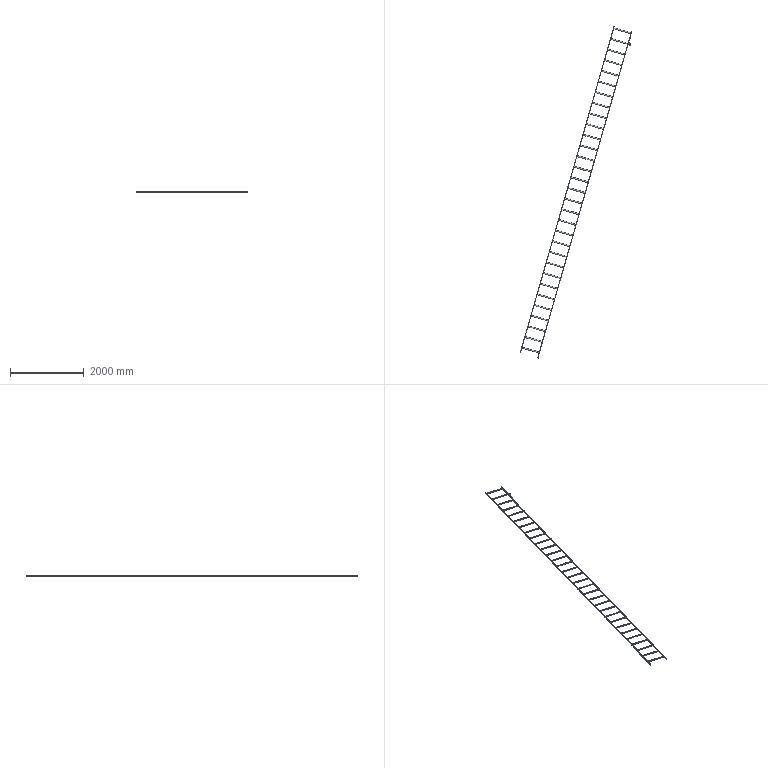Part | SolidWorks | features WeldMemberFeat 2, Chamfer 1, LPattern 1, Sweep 1, WeldCornerFeat 1, WeldmentFeature 1 | 34 solids | 213 faces | box 3019 x 8991 x 40 mm | volume 7846988 mm3 | cylinder 130 | plane 76 | torus 5 | cone 2 | commonest cylinder face diameters 20.8 x62 26.8 x62 12 x6